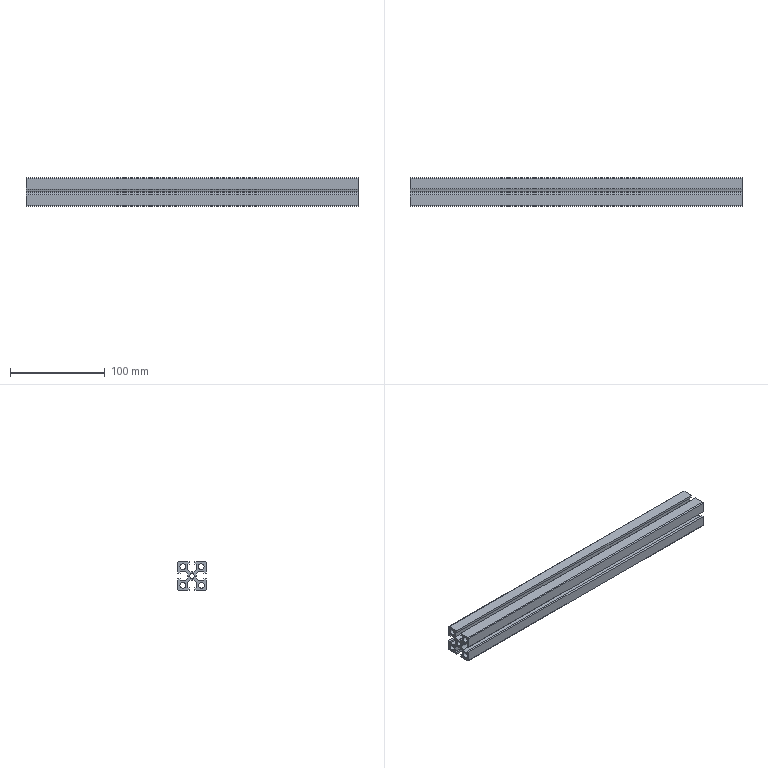Part | SolidWorks | features WeldMemberFeat 1, WeldmentFeature 1 | 1 solid | 64 faces | box 350 x 30 x 30 mm | volume 139651 mm3 | plane 42 | cylinder 22 | commonest cylinder face diameters 6 x8 15.262 x8 2 x4 5 x2